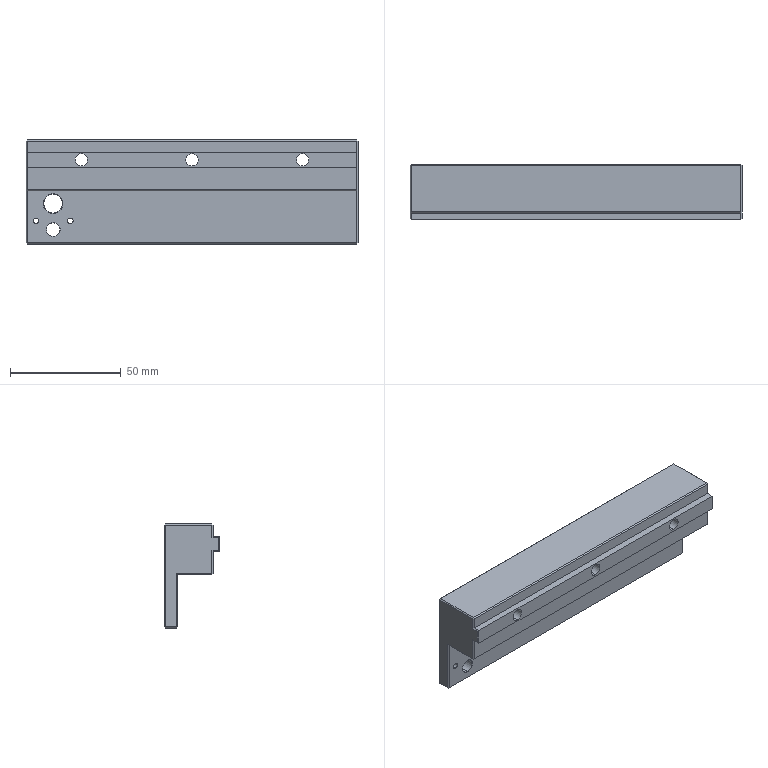Part | STEP file | BPSP-02-015 Fixture Locator V-Edge2_Default | 1 solid | 84 faces | box 150 x 25 x 47 mm | volume 97185 mm3 | plane 50 | cylinder 24 | cone 10 | commonest cylinder face diameters 2.5 x8 5.5 x6 10 x6 6 x2 8.5 x2